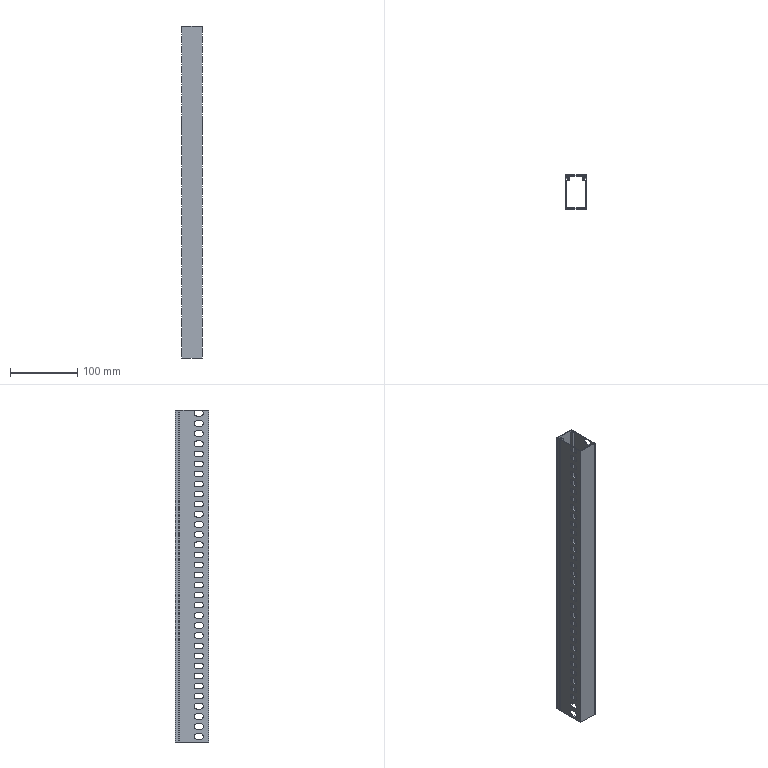Part | SolidWorks | features BaseBody 1 | 1 solid | 290 faces | box 30 x 50 x 493 mm | volume 80282 mm3 | plane 158 | cylinder 132 | commonest cylinder face diameters 8 x132